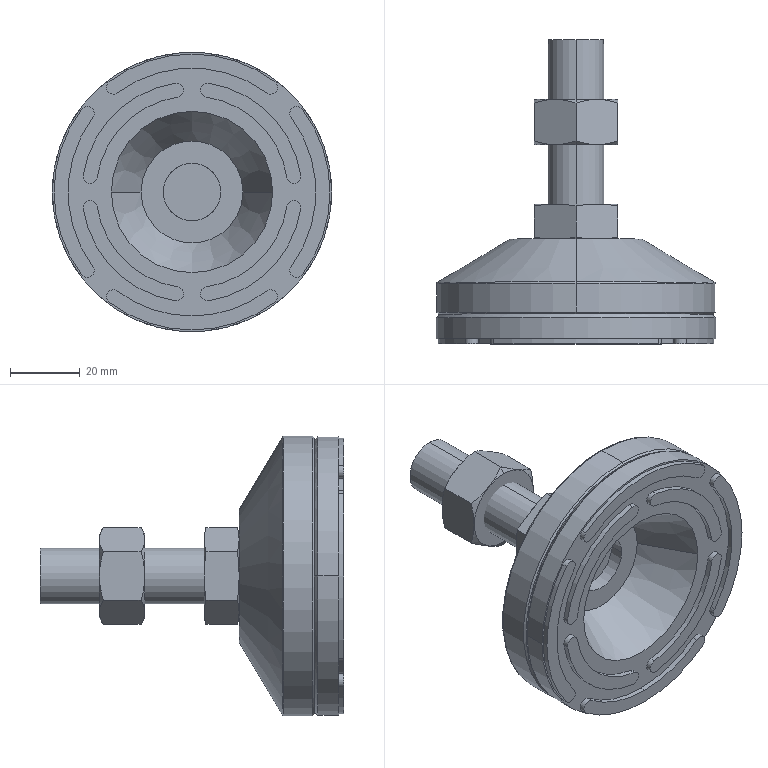Part | STEP file | E-WAC53-D80-M16-L100-1.STEP | 3 solids | 124 faces | box 80 x 87 x 80 mm | volume 91513 mm3 | cylinder 56 | cone 34 | plane 32 | torus 2 | commonest cylinder face diameters 4 x24 71 x5 79 x5 16.5 x4 55 x4 63 x4